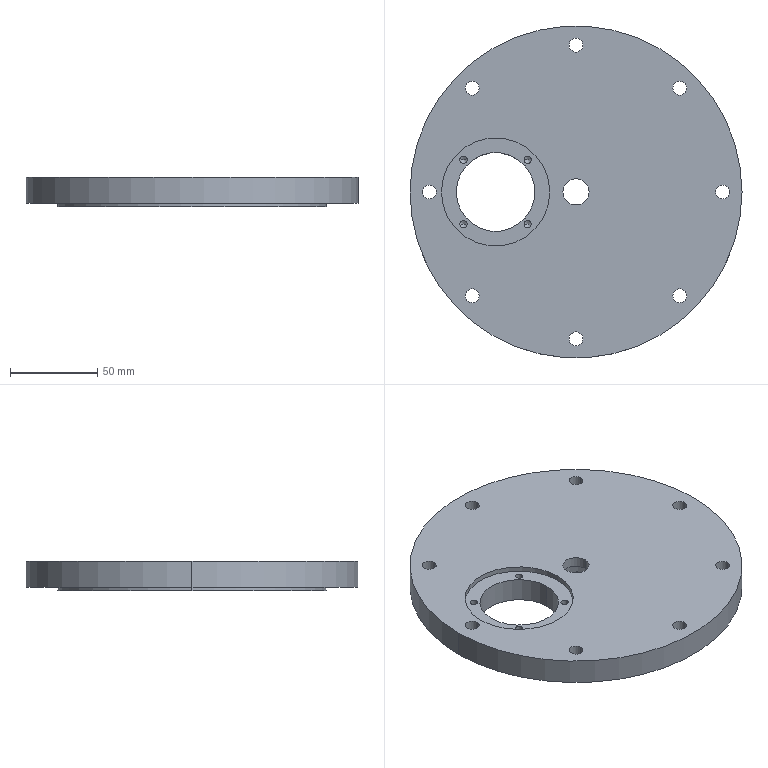Part | SolidWorks | features ICE 4, Cut 2, Extrusion 1, HoleWzd 1 | 1 solid | 49 faces | box 190 x 190 x 17 mm | volume 412970 mm3 | cylinder 36 | cone 8 | plane 5 | commonest cylinder face diameters 8 x16 4.2 x8 15 x2 35 x2 45 x2 62 x2
STEP:
#1=CARTESIAN_POINT('',(-4.,84.,-1484.048));
#2=VERTEX_POINT('',#1);
#3=CARTESIAN_POINT('',(4.,84.,-1484.048));
#4=VERTEX_POINT('',#3);
#5=CARTESIAN_POINT('',(0.,84.,-1484.048));
#6=DIRECTION('',(0.,0.,1.));
#7=DIRECTION('',(1.,0.,0.));
#8=AXIS2_PLACEMENT_3D('',#5,#6,#7);
#9=CIRCLE('',#8,4.);
#10=EDGE_CURVE('',#2,#4,#9,.T.);
#11=ORIENTED_EDGE('',*,*,#10,.F.);
#12=CARTESIAN_POINT('',(-4.,84.,-1469.048));
#13=VERTEX_POINT('',#12);
#14=CARTESIAN_POINT('',(-4.,84.,-1486.048));
#15=DIRECTION('',(0.,0.,1.));
#16=VECTOR('',#15,1000.);
#17=LINE('',#14,#16);
#18=EDGE_CURVE('',#2,#13,#17,.T.);
#19=ORIENTED_EDGE('',*,*,#18,.T.);
#20=CARTESIAN_POINT('',(4.,84.,-1469.048));
#21=VERTEX_POINT('',#20);
#22=CARTESIAN_POINT('',(0.,84.,-1469.048));
#23=DIRECTION('',(0.,0.,1.));
#24=DIRECTION('',(1.,0.,0.));
#25=AXIS2_PLACEMENT_3D('',#22,#23,#24);
#26=CIRCLE('',#25,4.);
#27=EDGE_CURVE('',#13,#21,#26,.T.);
#28=ORIENTED_EDGE('',*,*,#27,.T.);
#29=CARTESIAN_POINT('',(4.,84.,-1486.048));
#30=DIRECTION('',(0.,0.,1.));
#31=VECTOR('',#30,1000.);
#32=LINE('',#29,#31);
#33=EDGE_CURVE('',#4,#21,#32,.T.);
#34=ORIENTED_EDGE('',*,*,#33,.F.);
#35=EDGE_LOOP('',(#11,#19,#28,#34));
#36=FACE_OUTER_BOUND('',#35,.T.);
#37=CARTESIAN_POINT('',(0.,84.,-1486.048));
#38=DIRECTION('',(0.,0.,1.));
#39=DIRECTION('',(1.,0.,0.));
#40=AXIS2_PLACEMENT_3D('',#37,#38,#39);
#41=CYLINDRICAL_SURFACE('',#40,4.);
#42=ADVANCED_FACE('',(#36),#41,.F.);
#43=CARTESIAN_POINT('',(55.397,59.397,-1484.048));
#44=VERTEX_POINT('',#43);
#45=CARTESIAN_POINT('',(63.397,59.397,-1484.048));
#46=VERTEX_POINT('',#45);
#47=CARTESIAN_POINT('',(59.397,59.397,-1484.048));
#48=DIRECTION('',(0.,0.,1.));
#49=DIRECTION('',(1.,0.,0.));
#50=AXIS2_PLACEMENT_3D('',#47,#48,#49);
#51=CIRCLE('',#50,4.);
#52=EDGE_CURVE('',#44,#46,#51,.T.);
#53=ORIENTED_EDGE('',*,*,#52,.F.);
#54=CARTESIAN_POINT('',(55.397,59.397,-1469.048));
#55=VERTEX_POINT('',#54);
#56=CARTESIAN_POINT('',(55.397,59.397,-1486.048));
#57=DIRECTION('',(0.,0.,1.));
#58=VECTOR('',#57,1000.);
#59=LINE('',#56,#58);
#60=EDGE_CURVE('',#44,#55,#59,.T.);
#61=ORIENTED_EDGE('',*,*,#60,.T.);
#62=CARTESIAN_POINT('',(63.397,59.397,-1469.048));
#63=VERTEX_POINT('',#62);
#64=CARTESIAN_POINT('',(59.397,59.397,-1469.048));
#65=DIRECTION('',(0.,0.,1.));
#66=DIRECTION('',(1.,0.,0.));
#67=AXIS2_PLACEMENT_3D('',#64,#65,#66);
#68=CIRCLE('',#67,4.);
#69=EDGE_CURVE('',#55,#63,#68,.T.);
#70=ORIENTED_EDGE('',*,*,#69,.T.);
#71=CARTESIAN_POINT('',(63.397,59.397,-1486.048));
#72=DIRECTION('',(0.,0.,1.));
#73=VECTOR('',#72,1000.);
#74=LINE('',#71,#73);
#75=EDGE_CURVE('',#46,#63,#74,.T.);
#76=ORIENTED_EDGE('',*,*,#75,.F.);
#77=EDGE_LOOP('',(#53,#61,#70,#76));
#78=FACE_OUTER_BOUND('',#77,.T.);
#79=CARTESIAN_POINT('',(59.397,59.397,-1486.048));
#80=DIRECTION('',(0.,0.,1.));
#81=DIRECTION('',(1.,0.,0.));
#82=AXIS2_PLACEMENT_3D('',#79,#80,#81);
#83=CYLINDRICAL_SURFACE('',#82,4.);
#84=ADVANCED_FACE('',(#78),#83,.F.);
#85=CARTESIAN_POINT('',(80.,0.,-1484.048));
#86=VERTEX_POINT('',#85);
#87=CARTESIAN_POINT('',(88.,0.,-1484.048));
#88=VERTEX_POINT('',#87);
#89=CARTESIAN_POINT('',(84.,0.,-1484.048));
#90=DIRECTION('',(0.,0.,1.));
#91=DIRECTION('',(1.,0.,0.));
#92=AXIS2_PLACEMENT_3D('',#89,#90,#91);
#93=CIRCLE('',#92,4.);
#94=EDGE_CURVE('',#86,#88,#93,.T.);
#95=ORIENTED_EDGE('',*,*,#94,.F.);
#96=CARTESIAN_POINT('',(80.,0.,-1469.048));
#97=VERTEX_POINT('',#96);
#98=CARTESIAN_POINT('',(80.,0.,-1486.048));
#99=DIRECTION('',(0.,0.,1.));
#100=VECTOR('',#99,1000.);
#101=LINE('',#98,#100);
#102=EDGE_CURVE('',#86,#97,#101,.T.);
#103=ORIENTED_EDGE('',*,*,#102,.T.);
#104=CARTESIAN_POINT('',(88.,0.,-1469.048));
#105=VERTEX_POINT('',#104);
#106=CARTESIAN_POINT('',(84.,0.,-1469.048));
#107=DIRECTION('',(0.,0.,1.));
#108=DIRECTION('',(1.,0.,0.));
#109=AXIS2_PLACEMENT_3D('',#106,#107,#108);
#110=CIRCLE('',#109,4.);
#111=EDGE_CURVE('',#97,#105,#110,.T.);
#112=ORIENTED_EDGE('',*,*,#111,.T.);
#113=CARTESIAN_POINT('',(88.,0.,-1486.048));
#114=DIRECTION('',(0.,0.,1.));
#115=VECTOR('',#114,1000.);
#116=LINE('',#113,#115);
#117=EDGE_CURVE('',#88,#105,#116,.T.);
#118=ORIENTED_EDGE('',*,*,#117,.F.);
#119=EDGE_LOOP('',(#95,#103,#112,#118));
#120=FACE_OUTER_BOUND('',#119,.T.);
#121=CARTESIAN_POINT('',(84.,0.,-1486.048));
#122=DIRECTION('',(0.,0.,1.));
#123=DIRECTION('',(1.,0.,0.));
#124=AXIS2_PLACEMENT_3D('',#121,#122,#123);
#125=CYLINDRICAL_SURFACE('',#124,4.);
#126=ADVANCED_FACE('',(#120),#125,.F.);
#127=CARTESIAN_POINT('',(55.397,-59.397,-1484.048));
#128=VERTEX_POINT('',#127);
#129=CARTESIAN_POINT('',(63.397,-59.397,-1484.048));
#130=VERTEX_POINT('',#129);
#131=CARTESIAN_POINT('',(59.397,-59.397,-1484.048));
#132=DIRECTION('',(0.,0.,1.));
#133=DIRECTION('',(1.,0.,0.));
#134=AXIS2_PLACEMENT_3D('',#131,#132,#133);
#135=CIRCLE('',#134,4.);
#136=EDGE_CURVE('',#128,#130,#135,.T.);
#137=ORIENTED_EDGE('',*,*,#136,.F.);
#138=CARTESIAN_POINT('',(55.397,-59.397,-1469.048));
#139=VERTEX_POINT('',#138);
#140=CARTESIAN_POINT('',(55.397,-59.397,-1486.048));
#141=DIRECTION('',(0.,0.,1.));
#142=VECTOR('',#141,1000.);
#143=LINE('',#140,#142);
#144=EDGE_CURVE('',#128,#139,#143,.T.);
#145=ORIENTED_EDGE('',*,*,#144,.T.);
#146=CARTESIAN_POINT('',(63.397,-59.397,-1469.048));
#147=VERTEX_POINT('',#146);
#148=CARTESIAN_POINT('',(59.397,-59.397,-1469.048));
#149=DIRECTION('',(0.,0.,1.));
#150=DIRECTION('',(1.,0.,0.));
#151=AXIS2_PLACEMENT_3D('',#148,#149,#150);
#152=CIRCLE('',#151,4.);
#153=EDGE_CURVE('',#139,#147,#152,.T.);
#154=ORIENTED_EDGE('',*,*,#153,.T.);
#155=CARTESIAN_POINT('',(63.397,-59.397,-1486.048));
#156=DIRECTION('',(0.,0.,1.));
#157=VECTOR('',#156,1000.);
#158=LINE('',#155,#157);
#159=EDGE_CURVE('',#130,#147,#158,.T.);
#160=ORIENTED_EDGE('',*,*,#159,.F.);
#161=EDGE_LOOP('',(#137,#145,#154,#160));
#162=FACE_OUTER_BOUND('',#161,.T.);
#163=CARTESIAN_POINT('',(59.397,-59.397,-1486.048));
#164=DIRECTION('',(0.,0.,1.));
#165=DIRECTION('',(1.,0.,0.));
#166=AXIS2_PLACEMENT_3D('',#163,#164,#165);
#167=CYLINDRICAL_SURFACE('',#166,4.);
#168=ADVANCED_FACE('',(#162),#167,.F.);
#169=CARTESIAN_POINT('',(-4.,-84.,-1484.048));
#170=VERTEX_POINT('',#169);
#171=CARTESIAN_POINT('',(4.,-84.,-1484.048));
#172=VERTEX_POINT('',#171);
#173=CARTESIAN_POINT('',(0.,-84.,-1484.048));
#174=DIRECTION('',(0.,0.,1.));
#175=DIRECTION('',(1.,0.,0.));
#176=AXIS2_PLACEMENT_3D('',#173,#174,#175);
#177=CIRCLE('',#176,4.);
#178=EDGE_CURVE('',#170,#172,#177,.T.);
#179=ORIENTED_EDGE('',*,*,#178,.F.);
#180=CARTESIAN_POINT('',(-4.,-84.,-1469.048));
#181=VERTEX_POINT('',#180);
#182=CARTESIAN_POINT('',(-4.,-84.,-1486.048));
#183=DIRECTION('',(0.,0.,1.));
#184=VECTOR('',#183,1000.);
#185=LINE('',#182,#184);
#186=EDGE_CURVE('',#170,#181,#185,.T.);
#187=ORIENTED_EDGE('',*,*,#186,.T.);
#188=CARTESIAN_POINT('',(4.,-84.,-1469.048));
#189=VERTEX_POINT('',#188);
#190=CARTESIAN_POINT('',(0.,-84.,-1469.048));
#191=DIRECTION('',(0.,0.,1.));
#192=DIRECTION('',(1.,0.,0.));
#193=AXIS2_PLACEMENT_3D('',#190,#191,#192);
#194=CIRCLE('',#193,4.);
#195=EDGE_CURVE('',#181,#189,#194,.T.);
#196=ORIENTED_EDGE('',*,*,#195,.T.);
#197=CARTESIAN_POINT('',(4.,-84.,-1486.048));
#198=DIRECTION('',(0.,0.,1.));
#199=VECTOR('',#198,1000.);
#200=LINE('',#197,#199);
#201=EDGE_CURVE('',#172,#189,#200,.T.);
#202=ORIENTED_EDGE('',*,*,#201,.F.);
#203=EDGE_LOOP('',(#179,#187,#196,#202));
#204=FACE_OUTER_BOUND('',#203,.T.);
#205=CARTESIAN_POINT('',(0.,-84.,-1486.048));
#206=DIRECTION('',(0.,0.,1.));
#207=DIRECTION('',(1.,0.,0.));
#208=AXIS2_PLACEMENT_3D('',#205,#206,#207);
#209=CYLINDRICAL_SURFACE('',#208,4.);
#210=ADVANCED_FACE('',(#204),#209,.F.);
#211=CARTESIAN_POINT('',(-63.397,-59.397,-1484.048));
#212=VERTEX_POINT('',#211);
#213=CARTESIAN_POINT('',(-55.397,-59.397,-1484.048));
#214=VERTEX_POINT('',#213);
#215=CARTESIAN_POINT('',(-59.397,-59.397,-1484.048));
#216=DIRECTION('',(0.,0.,1.));
#217=DIRECTION('',(1.,0.,0.));
#218=AXIS2_PLACEMENT_3D('',#215,#216,#217);
#219=CIRCLE('',#218,4.);
#220=EDGE_CURVE('',#212,#214,#219,.T.);
#221=ORIENTED_EDGE('',*,*,#220,.F.);
#222=CARTESIAN_POINT('',(-63.397,-59.397,-1469.048));
#223=VERTEX_POINT('',#222);
#224=CARTESIAN_POINT('',(-63.397,-59.397,-1486.048));
#225=DIRECTION('',(0.,0.,1.));
#226=VECTOR('',#225,1000.);
#227=LINE('',#224,#226);
#228=EDGE_CURVE('',#212,#223,#227,.T.);
#229=ORIENTED_EDGE('',*,*,#228,.T.);
#230=CARTESIAN_POINT('',(-55.397,-59.397,-1469.048));
#231=VERTEX_POINT('',#230);
#232=CARTESIAN_POINT('',(-59.397,-59.397,-1469.048));
#233=DIRECTION('',(0.,0.,1.));
#234=DIRECTION('',(1.,0.,0.));
#235=AXIS2_PLACEMENT_3D('',#232,#233,#234);
#236=CIRCLE('',#235,4.);
#237=EDGE_CURVE('',#223,#231,#236,.T.);
#238=ORIENTED_EDGE('',*,*,#237,.T.);
#239=CARTESIAN_POINT('',(-55.397,-59.397,-1486.048));
#240=DIRECTION('',(0.,0.,1.));
#241=VECTOR('',#240,1000.);
#242=LINE('',#239,#241);
#243=EDGE_CURVE('',#214,#231,#242,.T.);
#244=ORIENTED_EDGE('',*,*,#243,.F.);
#245=EDGE_LOOP('',(#221,#229,#238,#244));
#246=FACE_OUTER_BOUND('',#245,.T.);
#247=CARTESIAN_POINT('',(-59.397,-59.397,-1486.048));
#248=DIRECTION('',(0.,0.,1.));
#249=DIRECTION('',(1.,0.,0.));
#250=AXIS2_PLACEMENT_3D('',#247,#248,#249);
#251=CYLINDRICAL_SURFACE('',#250,4.);
#252=ADVANCED_FACE('',(#246),#251,.F.);
#253=CARTESIAN_POINT('',(-88.,0.,-1484.048));
#254=VERTEX_POINT('',#253);
#255=CARTESIAN_POINT('',(-80.,0.,-1484.048));
#256=VERTEX_POINT('',#255);
#257=CARTESIAN_POINT('',(-84.,0.,-1484.048));
#258=DIRECTION('',(0.,0.,1.));
#259=DIRECTION('',(1.,0.,0.));
#260=AXIS2_PLACEMENT_3D('',#257,#258,#259);
#261=CIRCLE('',#260,4.);
#262=EDGE_CURVE('',#254,#256,#261,.T.);
#263=ORIENTED_EDGE('',*,*,#262,.F.);
#264=CARTESIAN_POINT('',(-88.,0.,-1469.048));
#265=VERTEX_POINT('',#264);
#266=CARTESIAN_POINT('',(-88.,0.,-1486.048));
#267=DIRECTION('',(0.,0.,1.));
#268=VECTOR('',#267,1000.);
#269=LINE('',#266,#268);
#270=EDGE_CURVE('',#254,#265,#269,.T.);
#271=ORIENTED_EDGE('',*,*,#270,.T.);
#272=CARTESIAN_POINT('',(-80.,0.,-1469.048));
#273=VERTEX_POINT('',#272);
#274=CARTESIAN_POINT('',(-84.,0.,-1469.048));
#275=DIRECTION('',(0.,0.,1.));
#276=DIRECTION('',(1.,0.,0.));
#277=AXIS2_PLACEMENT_3D('',#274,#275,#276);
#278=CIRCLE('',#277,4.);
#279=EDGE_CURVE('',#265,#273,#278,.T.);
#280=ORIENTED_EDGE('',*,*,#279,.T.);
#281=CARTESIAN_POINT('',(-80.,0.,-1486.048));
#282=DIRECTION('',(0.,0.,1.));
#283=VECTOR('',#282,1000.);
#284=LINE('',#281,#283);
#285=EDGE_CURVE('',#256,#273,#284,.T.);
#286=ORIENTED_EDGE('',*,*,#285,.F.);
#287=EDGE_LOOP('',(#263,#271,#280,#286));
#288=FACE_OUTER_BOUND('',#287,.T.);
#289=CARTESIAN_POINT('',(-84.,0.,-1486.048));
#290=DIRECTION('',(0.,0.,1.));
#291=DIRECTION('',(1.,0.,0.));
#292=AXIS2_PLACEMENT_3D('',#289,#290,#291);
#293=CYLINDRICAL_SURFACE('',#292,4.);
#294=ADVANCED_FACE('',(#288),#293,.F.);
#295=CARTESIAN_POINT('',(-63.397,59.397,-1484.048));
#296=VERTEX_POINT('',#295);
#297=CARTESIAN_POINT('',(-55.397,59.397,-1484.048));
#298=VERTEX_POINT('',#297);
#299=CARTESIAN_POINT('',(-59.397,59.397,-1484.048));
#300=DIRECTION('',(0.,0.,1.));
#301=DIRECTION('',(1.,0.,0.));
#302=AXIS2_PLACEMENT_3D('',#299,#300,#301);
#303=CIRCLE('',#302,4.);
#304=EDGE_CURVE('',#296,#298,#303,.T.);
#305=ORIENTED_EDGE('',*,*,#304,.F.);
#306=CARTESIAN_POINT('',(-63.397,59.397,-1469.048));
#307=VERTEX_POINT('',#306);
#308=CARTESIAN_POINT('',(-63.397,59.397,-1486.048));
#309=DIRECTION('',(0.,0.,1.));
#310=VECTOR('',#309,1000.);
#311=LINE('',#308,#310);
#312=EDGE_CURVE('',#296,#307,#311,.T.);
#313=ORIENTED_EDGE('',*,*,#312,.T.);
#314=CARTESIAN_POINT('',(-55.397,59.397,-1469.048));
#315=VERTEX_POINT('',#314);
#316=CARTESIAN_POINT('',(-59.397,59.397,-1469.048));
#317=DIRECTION('',(0.,0.,1.));
#318=DIRECTION('',(1.,0.,0.));
#319=AXIS2_PLACEMENT_3D('',#316,#317,#318);
#320=CIRCLE('',#319,4.);
#321=EDGE_CURVE('',#307,#315,#320,.T.);
#322=ORIENTED_EDGE('',*,*,#321,.T.);
#323=CARTESIAN_POINT('',(-55.397,59.397,-1486.048));
#324=DIRECTION('',(0.,0.,1.));
#325=VECTOR('',#324,1000.);
#326=LINE('',#323,#325);
#327=EDGE_CURVE('',#298,#315,#326,.T.);
#328=ORIENTED_EDGE('',*,*,#327,.F.);
#329=EDGE_LOOP('',(#305,#313,#322,#328));
#330=FACE_OUTER_BOUND('',#329,.T.);
#331=CARTESIAN_POINT('',(-59.397,59.397,-1486.048));
#332=DIRECTION('',(0.,0.,1.));
#333=DIRECTION('',(1.,0.,0.));
#334=AXIS2_PLACEMENT_3D('',#331,#332,#333);
#335=CYLINDRICAL_SURFACE('',#334,4.);
#336=ADVANCED_FACE('',(#330),#335,.F.);
#337=CARTESIAN_POINT('',(-29.715,18.385,-1482.048));
#338=VERTEX_POINT('',#337);
#339=CARTESIAN_POINT('',(-25.515,18.385,-1482.048));
#340=VERTEX_POINT('',#339);
#341=CARTESIAN_POINT('',(-27.615,18.385,-1482.048));
#342=DIRECTION('',(0.,0.,1.));
#343=DIRECTION('',(1.,0.,0.));
#344=AXIS2_PLACEMENT_3D('',#341,#342,#343);
#345=CIRCLE('',#344,2.1);
#346=EDGE_CURVE('',#338,#340,#345,.T.);
#347=ORIENTED_EDGE('',*,*,#346,.F.);
#348=CARTESIAN_POINT('',(-29.715,18.385,-1472.048));
#349=VERTEX_POINT('',#348);
#350=CARTESIAN_POINT('',(-29.715,18.385,-1472.048));
#351=DIRECTION('',(0.,0.,1.));
#352=VECTOR('',#351,1000.);
#353=LINE('',#350,#352);
#354=EDGE_CURVE('',#338,#349,#353,.T.);
#355=ORIENTED_EDGE('',*,*,#354,.T.);
#356=CARTESIAN_POINT('',(-25.515,18.385,-1472.048));
#357=VERTEX_POINT('',#356);
#358=CARTESIAN_POINT('',(-27.615,18.385,-1472.048));
#359=DIRECTION('',(0.,0.,1.));
#360=DIRECTION('',(1.,0.,0.));
#361=AXIS2_PLACEMENT_3D('',#358,#359,#360);
#362=CIRCLE('',#361,2.1);
#363=EDGE_CURVE('',#349,#357,#362,.T.);
#364=ORIENTED_EDGE('',*,*,#363,.T.);
#365=CARTESIAN_POINT('',(-25.515,18.385,-1472.048));
#366=DIRECTION('',(0.,0.,1.));
#367=VECTOR('',#366,1000.);
#368=LINE('',#365,#367);
#369=EDGE_CURVE('',#340,#357,#368,.T.);
#370=ORIENTED_EDGE('',*,*,#369,.F.);
#371=EDGE_LOOP('',(#347,#355,#364,#370));
#372=FACE_OUTER_BOUND('',#371,.T.);
#373=CARTESIAN_POINT('',(-27.615,18.385,-1472.048));
#374=DIRECTION('',(0.,0.,1.));
#375=DIRECTION('',(1.,0.,0.));
#376=AXIS2_PLACEMENT_3D('',#373,#374,#375);
#377=CYLINDRICAL_SURFACE('',#376,2.1);
#378=ADVANCED_FACE('',(#372),#377,.F.);
#379=CARTESIAN_POINT('',(-27.615,18.385,-1483.31));
#380=VERTEX_POINT('',#379);
#381=CARTESIAN_POINT('',(-25.515,18.385,-1482.048));
#382=DIRECTION('',(0.8572,0.,0.515));
#383=VECTOR('',#382,1000.);
#384=LINE('',#381,#383);
#385=EDGE_CURVE('',#380,#340,#384,.T.);
#386=ORIENTED_EDGE('',*,*,#385,.F.);
#387=CARTESIAN_POINT('',(-29.715,18.385,-1482.048));
#388=DIRECTION('',(-0.8572,0.,0.515));
#389=VECTOR('',#388,1000.);
#390=LINE('',#387,#389);
#391=EDGE_CURVE('',#380,#338,#390,.T.);
#392=ORIENTED_EDGE('',*,*,#391,.T.);
#393=ORIENTED_EDGE('',*,*,#346,.T.);
#394=EDGE_LOOP('',(#386,#392,#393));
#395=FACE_OUTER_BOUND('',#394,.T.);
#396=CARTESIAN_POINT('',(-27.615,18.385,-1482.048));
#397=DIRECTION('',(0.,0.,1.));
#398=DIRECTION('',(1.,0.,0.));
#399=AXIS2_PLACEMENT_3D('',#396,#397,#398);
#400=CONICAL_SURFACE('',#399,2.1,1.03);
#401=ADVANCED_FACE('',(#395),#400,.F.);
#402=CARTESIAN_POINT('',(-29.715,-18.385,-1482.048));
#403=VERTEX_POINT('',#402);
#404=CARTESIAN_POINT('',(-25.515,-18.385,-1482.048));
#405=VERTEX_POINT('',#404);
#406=CARTESIAN_POINT('',(-27.615,-18.385,-1482.048));
#407=DIRECTION('',(0.,0.,1.));
#408=DIRECTION('',(1.,0.,0.));
#409=AXIS2_PLACEMENT_3D('',#406,#407,#408);
#410=CIRCLE('',#409,2.1);
#411=EDGE_CURVE('',#403,#405,#410,.T.);
#412=ORIENTED_EDGE('',*,*,#411,.F.);
#413=CARTESIAN_POINT('',(-29.715,-18.385,-1472.048));
#414=VERTEX_POINT('',#413);
#415=CARTESIAN_POINT('',(-29.715,-18.385,-1472.048));
#416=DIRECTION('',(0.,0.,1.));
#417=VECTOR('',#416,1000.);
#418=LINE('',#415,#417);
#419=EDGE_CURVE('',#403,#414,#418,.T.);
#420=ORIENTED_EDGE('',*,*,#419,.T.);
#421=CARTESIAN_POINT('',(-25.515,-18.385,-1472.048));
#422=VERTEX_POINT('',#421);
#423=CARTESIAN_POINT('',(-27.615,-18.385,-1472.048));
#424=DIRECTION('',(0.,0.,1.));
#425=DIRECTION('',(1.,0.,0.));
#426=AXIS2_PLACEMENT_3D('',#423,#424,#425);
#427=CIRCLE('',#426,2.1);
#428=EDGE_CURVE('',#414,#422,#427,.T.);
#429=ORIENTED_EDGE('',*,*,#428,.T.);
#430=CARTESIAN_POINT('',(-25.515,-18.385,-1472.048));
#431=DIRECTION('',(0.,0.,1.));
#432=VECTOR('',#431,1000.);
#433=LINE('',#430,#432);
#434=EDGE_CURVE('',#405,#422,#433,.T.);
#435=ORIENTED_EDGE('',*,*,#434,.F.);
#436=EDGE_LOOP('',(#412,#420,#429,#435));
#437=FACE_OUTER_BOUND('',#436,.T.);
#438=CARTESIAN_POINT('',(-27.615,-18.385,-1472.048));
#439=DIRECTION('',(0.,0.,1.));
#440=DIRECTION('',(1.,0.,0.));
#441=AXIS2_PLACEMENT_3D('',#438,#439,#440);
#442=CYLINDRICAL_SURFACE('',#441,2.1);
#443=ADVANCED_FACE('',(#437),#442,.F.);
#444=CARTESIAN_POINT('',(-27.615,-18.385,-1483.31));
#445=VERTEX_POINT('',#444);
#446=CARTESIAN_POINT('',(-25.515,-18.385,-1482.048));
#447=DIRECTION('',(0.8572,0.,0.515));
#448=VECTOR('',#447,1000.);
#449=LINE('',#446,#448);
#450=EDGE_CURVE('',#445,#405,#449,.T.);
#451=ORIENTED_EDGE('',*,*,#450,.F.);
#452=CARTESIAN_POINT('',(-29.715,-18.385,-1482.048));
#453=DIRECTION('',(-0.8572,0.,0.515));
#454=VECTOR('',#453,1000.);
#455=LINE('',#452,#454);
#456=EDGE_CURVE('',#445,#403,#455,.T.);
#457=ORIENTED_EDGE('',*,*,#456,.T.);
#458=ORIENTED_EDGE('',*,*,#411,.T.);
#459=EDGE_LOOP('',(#451,#457,#458));
#460=FACE_OUTER_BOUND('',#459,.T.);
#461=CARTESIAN_POINT('',(-27.615,-18.385,-1482.048));
#462=DIRECTION('',(0.,0.,1.));
#463=DIRECTION('',(1.,0.,0.));
#464=AXIS2_PLACEMENT_3D('',#461,#462,#463);
#465=CONICAL_SURFACE('',#464,2.1,1.03);
#466=ADVANCED_FACE('',(#460),#465,.F.);
#467=CARTESIAN_POINT('',(-66.485,-18.385,-1482.048));
#468=VERTEX_POINT('',#467);
#469=CARTESIAN_POINT('',(-62.285,-18.385,-1482.048));
#470=VERTEX_POINT('',#469);
#471=CARTESIAN_POINT('',(-64.385,-18.385,-1482.048));
#472=DIRECTION('',(0.,0.,1.));
#473=DIRECTION('',(1.,0.,0.));
#474=AXIS2_PLACEMENT_3D('',#471,#472,#473);
#475=CIRCLE('',#474,2.1);
#476=EDGE_CURVE('',#468,#470,#475,.T.);
#477=ORIENTED_EDGE('',*,*,#476,.F.);
#478=CARTESIAN_POINT('',(-66.485,-18.385,-1472.048));
#479=VERTEX_POINT('',#478);
#480=CARTESIAN_POINT('',(-66.485,-18.385,-1472.048));
#481=DIRECTION('',(0.,0.,1.));
#482=VECTOR('',#481,1000.);
#483=LINE('',#480,#482);
#484=EDGE_CURVE('',#468,#479,#483,.T.);
#485=ORIENTED_EDGE('',*,*,#484,.T.);
#486=CARTESIAN_POINT('',(-62.285,-18.385,-1472.048));
#487=VERTEX_POINT('',#486);
#488=CARTESIAN_POINT('',(-64.385,-18.385,-1472.048));
#489=DIRECTION('',(0.,0.,1.));
#490=DIRECTION('',(1.,0.,0.));
#491=AXIS2_PLACEMENT_3D('',#488,#489,#490);
#492=CIRCLE('',#491,2.1);
#493=EDGE_CURVE('',#479,#487,#492,.T.);
#494=ORIENTED_EDGE('',*,*,#493,.T.);
#495=CARTESIAN_POINT('',(-62.285,-18.385,-1472.048));
#496=DIRECTION('',(0.,0.,1.));
#497=VECTOR('',#496,1000.);
#498=LINE('',#495,#497);
#499=EDGE_CURVE('',#470,#487,#498,.T.);
#500=ORIENTED_EDGE('',*,*,#499,.F.);
#501=EDGE_LOOP('',(#477,#485,#494,#500));
#502=FACE_OUTER_BOUND('',#501,.T.);
#503=CARTESIAN_POINT('',(-64.385,-18.385,-1472.048));
#504=DIRECTION('',(0.,0.,1.));
#505=DIRECTION('',(1.,0.,0.));
#506=AXIS2_PLACEMENT_3D('',#503,#504,#505);
#507=CYLINDRICAL_SURFACE('',#506,2.1);
#508=ADVANCED_FACE('',(#502),#507,.F.);
#509=CARTESIAN_POINT('',(-64.385,-18.385,-1483.31));
#510=VERTEX_POINT('',#509);
#511=CARTESIAN_POINT('',(-62.285,-18.385,-1482.048));
#512=DIRECTION('',(0.8572,0.,0.515));
#513=VECTOR('',#512,1000.);
#514=LINE('',#511,#513);
#515=EDGE_CURVE('',#510,#470,#514,.T.);
#516=ORIENTED_EDGE('',*,*,#515,.F.);
#517=CARTESIAN_POINT('',(-66.485,-18.385,-1482.048));
#518=DIRECTION('',(-0.8572,0.,0.515));
#519=VECTOR('',#518,1000.);
#520=LINE('',#517,#519);
#521=EDGE_CURVE('',#510,#468,#520,.T.);
#522=ORIENTED_EDGE('',*,*,#521,.T.);
#523=ORIENTED_EDGE('',*,*,#476,.T.);
#524=EDGE_LOOP('',(#516,#522,#523));
#525=FACE_OUTER_BOUND('',#524,.T.);
#526=CARTESIAN_POINT('',(-64.385,-18.385,-1482.048));
#527=DIRECTION('',(0.,0.,1.));
#528=DIRECTION('',(1.,0.,0.));
#529=AXIS2_PLACEMENT_3D('',#526,#527,#528);
#530=CONICAL_SURFACE('',#529,2.1,1.03);
#531=ADVANCED_FACE('',(#525),#530,.F.);
#532=CARTESIAN_POINT('',(-66.485,18.385,-1482.048));
#533=VERTEX_POINT('',#532);
#534=CARTESIAN_POINT('',(-62.285,18.385,-1482.048));
#535=VERTEX_POINT('',#534);
#536=CARTESIAN_POINT('',(-64.385,18.385,-1482.048));
#537=DIRECTION('',(0.,0.,1.));
#538=DIRECTION('',(1.,0.,0.));
#539=AXIS2_PLACEMENT_3D('',#536,#537,#538);
#540=CIRCLE('',#539,2.1);
#541=EDGE_CURVE('',#533,#535,#540,.T.);
#542=ORIENTED_EDGE('',*,*,#541,.F.);
#543=CARTESIAN_POINT('',(-66.485,18.385,-1472.048));
#544=VERTEX_POINT('',#543);
#545=CARTESIAN_POINT('',(-66.485,18.385,-1472.048));
#546=DIRECTION('',(0.,0.,1.));
#547=VECTOR('',#546,1000.);
#548=LINE('',#545,#547);
#549=EDGE_CURVE('',#533,#544,#548,.T.);
#550=ORIENTED_EDGE('',*,*,#549,.T.);
#551=CARTESIAN_POINT('',(-62.285,18.385,-1472.048));
#552=VERTEX_POINT('',#551);
#553=CARTESIAN_POINT('',(-64.385,18.385,-1472.048));
#554=DIRECTION('',(0.,0.,1.));
#555=DIRECTION('',(1.,0.,0.));
#556=AXIS2_PLACEMENT_3D('',#553,#554,#555);
#557=CIRCLE('',#556,2.1);
#558=EDGE_CURVE('',#544,#552,#557,.T.);
#559=ORIENTED_EDGE('',*,*,#558,.T.);
#560=CARTESIAN_POINT('',(-62.285,18.385,-1472.048));
#561=DIRECTION('',(0.,0.,1.));
#562=VECTOR('',#561,1000.);
#563=LINE('',#560,#562);
#564=EDGE_CURVE('',#535,#552,#563,.T.);
#565=ORIENTED_EDGE('',*,*,#564,.F.);
#566=EDGE_LOOP('',(#542,#550,#559,#565));
#567=FACE_OUTER_BOUND('',#566,.T.);
#568=CARTESIAN_POINT('',(-64.385,18.385,-1472.048));
#569=DIRECTION('',(0.,0.,1.));
#570=DIRECTION('',(1.,0.,0.));
#571=AXIS2_PLACEMENT_3D('',#568,#569,#570);
#572=CYLINDRICAL_SURFACE('',#571,2.1);
#573=ADVANCED_FACE('',(#567),#572,.F.);
#574=CARTESIAN_POINT('',(-64.385,18.385,-1483.31));
#575=VERTEX_POINT('',#574);
#576=CARTESIAN_POINT('',(-62.285,18.385,-1482.048));
#577=DIRECTION('',(0.8572,0.,0.515));
#578=VECTOR('',#577,1000.);
#579=LINE('',#576,#578);
#580=EDGE_CURVE('',#575,#535,#579,.T.);
#581=ORIENTED_EDGE('',*,*,#580,.F.);
#582=CARTESIAN_POINT('',(-66.485,18.385,-1482.048));
#583=DIRECTION('',(-0.8572,0.,0.515));
#584=VECTOR('',#583,1000.);
#585=LINE('',#582,#584);
#586=EDGE_CURVE('',#575,#533,#585,.T.);
#587=ORIENTED_EDGE('',*,*,#586,.T.);
#588=ORIENTED_EDGE('',*,*,#541,.T.);
#589=EDGE_LOOP('',(#581,#587,#588));
#590=FACE_OUTER_BOUND('',#589,.T.);
#591=CARTESIAN_POINT('',(-64.385,18.385,-1482.048));
#592=DIRECTION('',(0.,0.,1.));
#593=DIRECTION('',(1.,0.,0.));
#594=AXIS2_PLACEMENT_3D('',#591,#592,#593);
#595=CONICAL_SURFACE('',#594,2.1,1.03);
#596=ADVANCED_FACE('',(#590),#595,.F.);
#597=CARTESIAN_POINT('',(-77.,0.,-1472.048));
#598=VERTEX_POINT('',#597);
#599=CARTESIAN_POINT('',(-15.,0.,-1472.048));
#600=VERTEX_POINT('',#599);
#601=CARTESIAN_POINT('',(-46.,0.,-1472.048));
#602=DIRECTION('',(0.,0.,1.));
#603=DIRECTION('',(1.,0.,0.));
#604=AXIS2_PLACEMENT_3D('',#601,#602,#603);
#605=CIRCLE('',#604,31.);
#606=EDGE_CURVE('',#598,#600,#605,.T.);
#607=ORIENTED_EDGE('',*,*,#606,.F.);
#608=CARTESIAN_POINT('',(-77.,0.,-1469.048));
#609=VERTEX_POINT('',#608);
#610=CARTESIAN_POINT('',(-77.,0.,-1472.048));
#611=DIRECTION('',(0.,0.,1.));
#612=VECTOR('',#611,1000.);
#613=LINE('',#610,#612);
#614=EDGE_CURVE('',#598,#609,#613,.T.);
#615=ORIENTED_EDGE('',*,*,#614,.T.);
#616=CARTESIAN_POINT('',(-15.,0.,-1469.048));
#617=VERTEX_POINT('',#616);
#618=CARTESIAN_POINT('',(-46.,0.,-1469.048));
#619=DIRECTION('',(0.,0.,1.));
#620=DIRECTION('',(1.,0.,0.));
#621=AXIS2_PLACEMENT_3D('',#618,#619,#620);
#622=CIRCLE('',#621,31.);
#623=EDGE_CURVE('',#609,#617,#622,.T.);
#624=ORIENTED_EDGE('',*,*,#623,.T.);
#625=CARTESIAN_POINT('',(-15.,0.,-1472.048));
#626=DIRECTION('',(0.,0.,1.));
#627=VECTOR('',#626,1000.);
#628=LINE('',#625,#627);
#629=EDGE_CURVE('',#600,#617,#628,.T.);
#630=ORIENTED_EDGE('',*,*,#629,.F.);
#631=EDGE_LOOP('',(#607,#615,#624,#630));
#632=FACE_OUTER_BOUND('',#631,.T.);
#633=CARTESIAN_POINT('',(-46.,0.,-1472.048));
#634=DIRECTION('',(0.,0.,1.));
#635=DIRECTION('',(1.,0.,0.));
#636=AXIS2_PLACEMENT_3D('',#633,#634,#635);
#637=CYLINDRICAL_SURFACE('',#636,31.);
#638=ADVANCED_FACE('',(#632),#637,.F.);
#639=CARTESIAN_POINT('',(-7.5,0.,-1469.048));
#640=VERTEX_POINT('',#639);
#641=CARTESIAN_POINT('',(7.5,0.,-1469.048));
#642=VERTEX_POINT('',#641);
#643=CARTESIAN_POINT('',(0.,0.,-1469.048));
#644=DIRECTION('',(0.,0.,1.));
#645=DIRECTION('',(1.,0.,0.));
#646=AXIS2_PLACEMENT_3D('',#643,#644,#645);
#647=CIRCLE('',#646,7.5);
#648=EDGE_CURVE('',#640,#642,#647,.T.);
#649=ORIENTED_EDGE('',*,*,#648,.T.);
#650=CARTESIAN_POINT('',(7.5,0.,-1475.048));
#651=VERTEX_POINT('',#650);
#652=CARTESIAN_POINT('',(7.5,0.,-1463.048));
#653=DIRECTION('',(0.,0.,-1.));
#654=VECTOR('',#653,1000.);
#655=LINE('',#652,#654);
#656=EDGE_CURVE('',#642,#651,#655,.T.);
#657=ORIENTED_EDGE('',*,*,#656,.T.);
#658=CARTESIAN_POINT('',(-7.5,0.,-1475.048));
#659=VERTEX_POINT('',#658);
#660=CARTESIAN_POINT('',(0.,0.,-1475.048));
#661=DIRECTION('',(0.,0.,-1.));
#662=DIRECTION('',(-1.,0.,0.));
#663=AXIS2_PLACEMENT_3D('',#660,#661,#662);
#664=CIRCLE('',#663,7.5);
#665=EDGE_CURVE('',#651,#659,#664,.T.);
#666=ORIENTED_EDGE('',*,*,#665,.T.);
#667=CARTESIAN_POINT('',(-7.5,0.,-1463.048));
#668=DIRECTION('',(0.,0.,-1.));
#669=VECTOR('',#668,1000.);
#670=LINE('',#667,#669);
#671=EDGE_CURVE('',#640,#659,#670,.T.);
#672=ORIENTED_EDGE('',*,*,#671,.F.);
#673=EDGE_LOOP('',(#649,#657,#666,#672));
#674=FACE_OUTER_BOUND('',#673,.T.);
#675=CARTESIAN_POINT('',(0.,0.,-1463.048));
#676=DIRECTION('',(0.,0.,-1.));
#677=DIRECTION('',(-1.,0.,0.));
#678=AXIS2_PLACEMENT_3D('',#675,#676,#677);
#679=CYLINDRICAL_SURFACE('',#678,7.5);
#680=ADVANCED_FACE('',(#674),#679,.F.);
#681=CARTESIAN_POINT('',(17.5,0.,-1475.048));
#682=VERTEX_POINT('',#681);
#683=CARTESIAN_POINT('',(-17.5,0.,-1475.048));
#684=VERTEX_POINT('',#683);
#685=CARTESIAN_POINT('',(0.,0.,-1475.048));
#686=DIRECTION('',(0.,0.,-1.));
#687=DIRECTION('',(-1.,0.,0.));
#688=AXIS2_PLACEMENT_3D('',#685,#686,#687);
#689=CIRCLE('',#688,17.5);
#690=EDGE_CURVE('',#682,#684,#689,.T.);
#691=ORIENTED_EDGE('',*,*,#690,.F.);
#692=CARTESIAN_POINT('',(17.5,0.,-1486.048));
#693=VERTEX_POINT('',#692);
#694=CARTESIAN_POINT('',(17.5,0.,-1475.048));
#695=DIRECTION('',(0.,0.,-1.));
#696=VECTOR('',#695,1000.);
#697=LINE('',#694,#696);
#698=EDGE_CURVE('',#682,#693,#697,.T.);
#699=ORIENTED_EDGE('',*,*,#698,.T.);
#700=CARTESIAN_POINT('',(-17.5,0.,-1486.048));
#701=VERTEX_POINT('',#700);
#702=CARTESIAN_POINT('',(0.,0.,-1486.048));
#703=DIRECTION('',(0.,0.,-1.));
#704=DIRECTION('',(-1.,0.,0.));
#705=AXIS2_PLACEMENT_3D('',#702,#703,#704);
#706=CIRCLE('',#705,17.5);
#707=EDGE_CURVE('',#693,#701,#706,.T.);
#708=ORIENTED_EDGE('',*,*,#707,.T.);
#709=CARTESIAN_POINT('',(-17.5,0.,-1475.048));
#710=DIRECTION('',(0.,0.,-1.));
#711=VECTOR('',#710,1000.);
#712=LINE('',#709,#711);
#713=EDGE_CURVE('',#684,#701,#712,.T.);
#714=ORIENTED_EDGE('',*,*,#713,.F.);
#715=EDGE_LOOP('',(#691,#699,#708,#714));
#716=FACE_OUTER_BOUND('',#715,.T.);
#717=CARTESIAN_POINT('',(0.,0.,-1475.048));
#718=DIRECTION('',(0.,0.,-1.));
#719=DIRECTION('',(-1.,0.,0.));
#720=AXIS2_PLACEMENT_3D('',#717,#718,#719);
#721=CYLINDRICAL_SURFACE('',#720,17.5);
#722=ADVANCED_FACE('',(#716),#721,.F.);
#723=CARTESIAN_POINT('',(-77.,0.,-1486.048));
#724=VERTEX_POINT('',#723);
#725=CARTESIAN_POINT('',(77.,0.,-1486.048));
#726=VERTEX_POINT('',#725);
#727=CARTESIAN_POINT('',(0.,0.,-1486.048));
#728=DIRECTION('',(0.,0.,-1.));
#729=DIRECTION('',(-1.,0.,0.));
#730=AXIS2_PLACEMENT_3D('',#727,#728,#729);
#731=CIRCLE('',#730,77.);
#732=EDGE_CURVE('',#724,#726,#731,.T.);
#733=ORIENTED_EDGE('',*,*,#732,.F.);
#734=CARTESIAN_POINT('',(-77.,0.,-1484.048));
#735=VERTEX_POINT('',#734);
#736=CARTESIAN_POINT('',(-77.,0.,-1486.048));
#737=DIRECTION('',(0.,0.,1.));
#738=VECTOR('',#737,1000.);
#739=LINE('',#736,#738);
#740=EDGE_CURVE('',#724,#735,#739,.T.);
#741=ORIENTED_EDGE('',*,*,#740,.T.);
#742=CARTESIAN_POINT('',(77.,0.,-1484.048));
#743=VERTEX_POINT('',#742);
#744=CARTESIAN_POINT('',(0.,0.,-1484.048));
#745=DIRECTION('',(0.,0.,-1.));
#746=DIRECTION('',(-1.,0.,0.));
#747=AXIS2_PLACEMENT_3D('',#744,#745,#746);
#748=CIRCLE('',#747,77.);
#749=EDGE_CURVE('',#735,#743,#748,.T.);
#750=ORIENTED_EDGE('',*,*,#749,.T.);
#751=CARTESIAN_POINT('',(77.,0.,-1486.048));
#752=DIRECTION('',(0.,0.,1.));
#753=VECTOR('',#752,1000.);
#754=LINE('',#751,#753);
#755=EDGE_CURVE('',#726,#743,#754,.T.);
#756=ORIENTED_EDGE('',*,*,#755,.F.);
#757=EDGE_LOOP('',(#733,#741,#750,#756));
#758=FACE_OUTER_BOUND('',#757,.T.);
#759=CARTESIAN_POINT('',(0.,0.,-1486.048));
#760=DIRECTION('',(0.,0.,1.));
#761=DIRECTION('',(1.,0.,0.));
#762=AXIS2_PLACEMENT_3D('',#759,#760,#761);
#763=CYLINDRICAL_SURFACE('',#762,77.);
#764=ADVANCED_FACE('',(#758),#763,.T.);
#765=CARTESIAN_POINT('',(95.,0.,-1469.048));
#766=VERTEX_POINT('',#765);
#767=CARTESIAN_POINT('',(-95.,0.,-1469.048));
#768=VERTEX_POINT('',#767);
#769=CARTESIAN_POINT('',(0.,0.,-1469.048));
#770=DIRECTION('',(0.,0.,1.));
#771=DIRECTION('',(1.,0.,0.));
#772=AXIS2_PLACEMENT_3D('',#769,#770,#771);
#773=CIRCLE('',#772,95.);
#774=EDGE_CURVE('',#766,#768,#773,.T.);
#775=ORIENTED_EDGE('',*,*,#774,.F.);
#776=CARTESIAN_POINT('',(95.,0.,-1484.048));
#777=VERTEX_POINT('',#776);
#778=CARTESIAN_POINT('',(95.,0.,-1469.048));
#779=DIRECTION('',(0.,0.,-1.));
#780=VECTOR('',#779,1000.);
#781=LINE('',#778,#780);
#782=EDGE_CURVE('',#766,#777,#781,.T.);
#783=ORIENTED_EDGE('',*,*,#782,.T.);
#784=CARTESIAN_POINT('',(-95.,0.,-1484.048));
#785=VERTEX_POINT('',#784);
#786=CARTESIAN_POINT('',(0.,0.,-1484.048));
#787=DIRECTION('',(0.,0.,1.));
#788=DIRECTION('',(1.,0.,0.));
#789=AXIS2_PLACEMENT_3D('',#786,#787,#788);
#790=CIRCLE('',#789,95.);
#791=EDGE_CURVE('',#777,#785,#790,.T.);
#792=ORIENTED_EDGE('',*,*,#791,.T.);
#793=CARTESIAN_POINT('',(-95.,0.,-1469.048));
#794=DIRECTION('',(0.,0.,-1.));
#795=VECTOR('',#794,1000.);
#796=LINE('',#793,#795);
#797=EDGE_CURVE('',#768,#785,#796,.T.);
#798=ORIENTED_EDGE('',*,*,#797,.F.);
#799=EDGE_LOOP('',(#775,#783,#792,#798));
#800=FACE_OUTER_BOUND('',#799,.T.);
#801=CARTESIAN_POINT('',(0.,0.,-1469.048));
#802=DIRECTION('',(0.,0.,-1.));
#803=DIRECTION('',(-1.,0.,0.));
#804=AXIS2_PLACEMENT_3D('',#801,#802,#803);
#805=CYLINDRICAL_SURFACE('',#804,95.);
#806=ADVANCED_FACE('',(#800),#805,.T.);
#807=CARTESIAN_POINT('',(-68.5,0.,-1486.048));
#808=VERTEX_POINT('',#807);
#809=CARTESIAN_POINT('',(-23.5,0.,-1486.048));
#810=VERTEX_POINT('',#809);
#811=CARTESIAN_POINT('',(-46.,0.,-1486.048));
#812=DIRECTION('',(0.,0.,1.));
#813=DIRECTION('',(1.,0.,0.));
#814=AXIS2_PLACEMENT_3D('',#811,#812,#813);
#815=CIRCLE('',#814,22.5);
#816=EDGE_CURVE('',#808,#810,#815,.T.);
#817=ORIENTED_EDGE('',*,*,#816,.F.);
#818=CARTESIAN_POINT('',(-68.5,0.,-1472.048));
#819=VERTEX_POINT('',#818);
#820=CARTESIAN_POINT('',(-68.5,0.,-1486.048));
#821=DIRECTION('',(0.,0.,1.));
#822=VECTOR('',#821,1000.);
#823=LINE('',#820,#822);
#824=EDGE_CURVE('',#808,#819,#823,.T.);
#825=ORIENTED_EDGE('',*,*,#824,.T.);
#826=CARTESIAN_POINT('',(-23.5,0.,-1472.048));
#827=VERTEX_POINT('',#826);
#828=CARTESIAN_POINT('',(-46.,0.,-1472.048));
#829=DIRECTION('',(0.,0.,-1.));
#830=DIRECTION('',(1.,0.,0.));
#831=AXIS2_PLACEMENT_3D('',#828,#829,#830);
#832=CIRCLE('',#831,22.5);
#833=EDGE_CURVE('',#827,#819,#832,.T.);
#834=ORIENTED_EDGE('',*,*,#833,.F.);
#835=CARTESIAN_POINT('',(-23.5,0.,-1486.048));
#836=DIRECTION('',(0.,0.,1.));
#837=VECTOR('',#836,1000.);
#838=LINE('',#835,#837);
#839=EDGE_CURVE('',#810,#827,#838,.T.);
#840=ORIENTED_EDGE('',*,*,#839,.F.);
#841=EDGE_LOOP('',(#817,#825,#834,#840));
#842=FACE_OUTER_BOUND('',#841,.T.);
#843=CARTESIAN_POINT('',(-46.,0.,-1486.048));
#844=DIRECTION('',(0.,0.,1.));
#845=DIRECTION('',(1.,0.,0.));
#846=AXIS2_PLACEMENT_3D('',#843,#844,#845);
#847=CYLINDRICAL_SURFACE('',#846,22.5);
#848=ADVANCED_FACE('',(#842),#847,.F.);
#849=ORIENTED_EDGE('',*,*,#824,.F.);
#850=CARTESIAN_POINT('',(-46.,0.,-1486.048));
#851=DIRECTION('',(0.,0.,1.));
#852=DIRECTION('',(1.,0.,0.));
#853=AXIS2_PLACEMENT_3D('',#850,#851,#852);
#854=CIRCLE('',#853,22.5);
#855=EDGE_CURVE('',#810,#808,#854,.T.);
#856=ORIENTED_EDGE('',*,*,#855,.F.);
#857=ORIENTED_EDGE('',*,*,#839,.T.);
#858=CARTESIAN_POINT('',(-46.,0.,-1472.048));
#859=DIRECTION('',(0.,0.,-1.));
#860=DIRECTION('',(1.,0.,0.));
#861=AXIS2_PLACEMENT_3D('',#858,#859,#860);
#862=CIRCLE('',#861,22.5);
#863=EDGE_CURVE('',#819,#827,#862,.T.);
#864=ORIENTED_EDGE('',*,*,#863,.F.);
#865=EDGE_LOOP('',(#849,#856,#857,#864));
#866=FACE_OUTER_BOUND('',#865,.T.);
#867=CARTESIAN_POINT('',(-46.,0.,-1486.048));
#868=DIRECTION('',(0.,0.,1.));
#869=DIRECTION('',(1.,0.,0.));
#870=AXIS2_PLACEMENT_3D('',#867,#868,#869);
#871=CYLINDRICAL_SURFACE('',#870,22.5);
#872=ADVANCED_FACE('',(#866),#871,.F.);
#873=ORIENTED_EDGE('',*,*,#782,.F.);
#874=CARTESIAN_POINT('',(0.,0.,-1469.048));
#875=DIRECTION('',(0.,0.,1.));
#876=DIRECTION('',(1.,0.,0.));
#877=AXIS2_PLACEMENT_3D('',#874,#875,#876);
#878=CIRCLE('',#877,95.);
#879=EDGE_CURVE('',#768,#766,#878,.T.);
#880=ORIENTED_EDGE('',*,*,#879,.F.);
#881=ORIENTED_EDGE('',*,*,#797,.T.);
#882=CARTESIAN_POINT('',(0.,0.,-1484.048));
#883=DIRECTION('',(0.,0.,1.));
#884=DIRECTION('',(1.,0.,0.));
#885=AXIS2_PLACEMENT_3D('',#882,#883,#884);
#886=CIRCLE('',#885,95.);
#887=EDGE_CURVE('',#785,#777,#886,.T.);
#888=ORIENTED_EDGE('',*,*,#887,.T.);
#889=EDGE_LOOP('',(#873,#880,#881,#888));
#890=FACE_OUTER_BOUND('',#889,.T.);
#891=CARTESIAN_POINT('',(0.,0.,-1469.048));
#892=DIRECTION('',(0.,0.,-1.));
#893=DIRECTION('',(-1.,0.,0.));
#894=AXIS2_PLACEMENT_3D('',#891,#892,#893);
#895=CYLINDRICAL_SURFACE('',#894,95.);
#896=ADVANCED_FACE('',(#890),#895,.T.);
#897=CARTESIAN_POINT('',(0.,84.,-1469.048));
#898=DIRECTION('',(0.,0.,1.));
#899=DIRECTION('',(1.,0.,0.));
#900=AXIS2_PLACEMENT_3D('',#897,#898,#899);
#901=CIRCLE('',#900,4.);
#902=EDGE_CURVE('',#21,#13,#901,.T.);
#903=ORIENTED_EDGE('',*,*,#902,.F.);
#904=ORIENTED_EDGE('',*,*,#27,.F.);
#905=EDGE_LOOP('',(#903,#904));
#906=FACE_BOUND('',#905,.T.);
#907=CARTESIAN_POINT('',(59.397,59.397,-1469.048));
#908=DIRECTION('',(0.,0.,1.));
#909=DIRECTION('',(1.,0.,0.));
#910=AXIS2_PLACEMENT_3D('',#907,#908,#909);
#911=CIRCLE('',#910,4.);
#912=EDGE_CURVE('',#63,#55,#911,.T.);
#913=ORIENTED_EDGE('',*,*,#912,.F.);
#914=ORIENTED_EDGE('',*,*,#69,.F.);
#915=EDGE_LOOP('',(#913,#914));
#916=FACE_BOUND('',#915,.T.);
#917=CARTESIAN_POINT('',(84.,0.,-1469.048));
#918=DIRECTION('',(0.,0.,1.));
#919=DIRECTION('',(1.,0.,0.));
#920=AXIS2_PLACEMENT_3D('',#917,#918,#919);
#921=CIRCLE('',#920,4.);
#922=EDGE_CURVE('',#105,#97,#921,.T.);
#923=ORIENTED_EDGE('',*,*,#922,.F.);
#924=ORIENTED_EDGE('',*,*,#111,.F.);
#925=EDGE_LOOP('',(#923,#924));
#926=FACE_BOUND('',#925,.T.);
#927=CARTESIAN_POINT('',(59.397,-59.397,-1469.048));
#928=DIRECTION('',(0.,0.,1.));
#929=DIRECTION('',(1.,0.,0.));
#930=AXIS2_PLACEMENT_3D('',#927,#928,#929);
#931=CIRCLE('',#930,4.);
#932=EDGE_CURVE('',#147,#139,#931,.T.);
#933=ORIENTED_EDGE('',*,*,#932,.F.);
#934=ORIENTED_EDGE('',*,*,#153,.F.);
#935=EDGE_LOOP('',(#933,#934));
#936=FACE_BOUND('',#935,.T.);
#937=CARTESIAN_POINT('',(0.,-84.,-1469.048));
#938=DIRECTION('',(0.,0.,1.));
#939=DIRECTION('',(1.,0.,0.));
#940=AXIS2_PLACEMENT_3D('',#937,#938,#939);
#941=CIRCLE('',#940,4.);
#942=EDGE_CURVE('',#189,#181,#941,.T.);
#943=ORIENTED_EDGE('',*,*,#942,.F.);
#944=ORIENTED_EDGE('',*,*,#195,.F.);
#945=EDGE_LOOP('',(#943,#944));
#946=FACE_BOUND('',#945,.T.);
#947=CARTESIAN_POINT('',(-59.397,-59.397,-1469.048));
#948=DIRECTION('',(0.,0.,1.));
#949=DIRECTION('',(1.,0.,0.));
#950=AXIS2_PLACEMENT_3D('',#947,#948,#949);
#951=CIRCLE('',#950,4.);
#952=EDGE_CURVE('',#231,#223,#951,.T.);
#953=ORIENTED_EDGE('',*,*,#952,.F.);
#954=ORIENTED_EDGE('',*,*,#237,.F.);
#955=EDGE_LOOP('',(#953,#954));
#956=FACE_BOUND('',#955,.T.);
#957=CARTESIAN_POINT('',(-84.,0.,-1469.048));
#958=DIRECTION('',(0.,0.,1.));
#959=DIRECTION('',(1.,0.,0.));
#960=AXIS2_PLACEMENT_3D('',#957,#958,#959);
#961=CIRCLE('',#960,4.);
#962=EDGE_CURVE('',#273,#265,#961,.T.);
#963=ORIENTED_EDGE('',*,*,#962,.F.);
#964=ORIENTED_EDGE('',*,*,#279,.F.);
#965=EDGE_LOOP('',(#963,#964));
#966=FACE_BOUND('',#965,.T.);
#967=CARTESIAN_POINT('',(-59.397,59.397,-1469.048));
#968=DIRECTION('',(0.,0.,1.));
#969=DIRECTION('',(1.,0.,0.));
#970=AXIS2_PLACEMENT_3D('',#967,#968,#969);
#971=CIRCLE('',#970,4.);
#972=EDGE_CURVE('',#315,#307,#971,.T.);
#973=ORIENTED_EDGE('',*,*,#972,.F.);
#974=ORIENTED_EDGE('',*,*,#321,.F.);
#975=EDGE_LOOP('',(#973,#974));
#976=FACE_BOUND('',#975,.T.);
#977=CARTESIAN_POINT('',(-46.,0.,-1469.048));
#978=DIRECTION('',(0.,0.,1.));
#979=DIRECTION('',(1.,0.,0.));
#980=AXIS2_PLACEMENT_3D('',#977,#978,#979);
#981=CIRCLE('',#980,31.);
#982=EDGE_CURVE('',#617,#609,#981,.T.);
#983=ORIENTED_EDGE('',*,*,#982,.F.);
#984=ORIENTED_EDGE('',*,*,#623,.F.);
#985=EDGE_LOOP('',(#983,#984));
#986=FACE_BOUND('',#985,.T.);
#987=ORIENTED_EDGE('',*,*,#648,.F.);
#988=CARTESIAN_POINT('',(0.,0.,-1469.048));
#989=DIRECTION('',(0.,0.,1.));
#990=DIRECTION('',(1.,0.,0.));
#991=AXIS2_PLACEMENT_3D('',#988,#989,#990);
#992=CIRCLE('',#991,7.5);
#993=EDGE_CURVE('',#642,#640,#992,.T.);
#994=ORIENTED_EDGE('',*,*,#993,.F.);
#995=EDGE_LOOP('',(#987,#994));
#996=FACE_BOUND('',#995,.T.);
#997=ORIENTED_EDGE('',*,*,#879,.T.);
#998=ORIENTED_EDGE('',*,*,#774,.T.);
#999=EDGE_LOOP('',(#997,#998));
#1000=FACE_OUTER_BOUND('',#999,.T.);
#1001=CARTESIAN_POINT('',(0.,0.,-1469.048));
#1002=DIRECTION('',(0.,0.,1.));
#1003=DIRECTION('',(1.,0.,0.));
#1004=AXIS2_PLACEMENT_3D('',#1001,#1002,#1003);
#1005=PLANE('',#1004);
#1006=ADVANCED_FACE('',(#906,#916,#926,#936,#946,#956,#966,#976,#986,#996,#1000),#1005,.T.);
#1007=CARTESIAN_POINT('',(0.,84.,-1484.048));
#1008=DIRECTION('',(0.,0.,1.));
#1009=DIRECTION('',(1.,0.,0.));
#1010=AXIS2_PLACEMENT_3D('',#1007,#1008,#1009);
#1011=CIRCLE('',#1010,4.);
#1012=EDGE_CURVE('',#4,#2,#1011,.T.);
#1013=ORIENTED_EDGE('',*,*,#1012,.T.);
#1014=ORIENTED_EDGE('',*,*,#10,.T.);
#1015=EDGE_LOOP('',(#1013,#1014));
#1016=FACE_BOUND('',#1015,.T.);
#1017=CARTESIAN_POINT('',(59.397,59.397,-1484.048));
#1018=DIRECTION('',(0.,0.,1.));
#1019=DIRECTION('',(1.,0.,0.));
#1020=AXIS2_PLACEMENT_3D('',#1017,#1018,#1019);
#1021=CIRCLE('',#1020,4.);
#1022=EDGE_CURVE('',#46,#44,#1021,.T.);
#1023=ORIENTED_EDGE('',*,*,#1022,.T.);
#1024=ORIENTED_EDGE('',*,*,#52,.T.);
#1025=EDGE_LOOP('',(#1023,#1024));
#1026=FACE_BOUND('',#1025,.T.);
#1027=CARTESIAN_POINT('',(84.,0.,-1484.048));
#1028=DIRECTION('',(0.,0.,1.));
#1029=DIRECTION('',(1.,0.,0.));
#1030=AXIS2_PLACEMENT_3D('',#1027,#1028,#1029);
#1031=CIRCLE('',#1030,4.);
#1032=EDGE_CURVE('',#88,#86,#1031,.T.);
#1033=ORIENTED_EDGE('',*,*,#1032,.T.);
#1034=ORIENTED_EDGE('',*,*,#94,.T.);
#1035=EDGE_LOOP('',(#1033,#1034));
#1036=FACE_BOUND('',#1035,.T.);
#1037=CARTESIAN_POINT('',(59.397,-59.397,-1484.048));
#1038=DIRECTION('',(0.,0.,1.));
#1039=DIRECTION('',(1.,0.,0.));
#1040=AXIS2_PLACEMENT_3D('',#1037,#1038,#1039);
#1041=CIRCLE('',#1040,4.);
#1042=EDGE_CURVE('',#130,#128,#1041,.T.);
#1043=ORIENTED_EDGE('',*,*,#1042,.T.);
#1044=ORIENTED_EDGE('',*,*,#136,.T.);
#1045=EDGE_LOOP('',(#1043,#1044));
#1046=FACE_BOUND('',#1045,.T.);
#1047=CARTESIAN_POINT('',(0.,-84.,-1484.048));
#1048=DIRECTION('',(0.,0.,1.));
#1049=DIRECTION('',(1.,0.,0.));
#1050=AXIS2_PLACEMENT_3D('',#1047,#1048,#1049);
#1051=CIRCLE('',#1050,4.);
#1052=EDGE_CURVE('',#172,#170,#1051,.T.);
#1053=ORIENTED_EDGE('',*,*,#1052,.T.);
#1054=ORIENTED_EDGE('',*,*,#178,.T.);
#1055=EDGE_LOOP('',(#1053,#1054));
#1056=FACE_BOUND('',#1055,.T.);
#1057=CARTESIAN_POINT('',(-59.397,-59.397,-1484.048));
#1058=DIRECTION('',(0.,0.,1.));
#1059=DIRECTION('',(1.,0.,0.));
#1060=AXIS2_PLACEMENT_3D('',#1057,#1058,#1059);
#1061=CIRCLE('',#1060,4.);
#1062=EDGE_CURVE('',#214,#212,#1061,.T.);
#1063=ORIENTED_EDGE('',*,*,#1062,.T.);
#1064=ORIENTED_EDGE('',*,*,#220,.T.);
#1065=EDGE_LOOP('',(#1063,#1064));
#1066=FACE_BOUND('',#1065,.T.);
#1067=CARTESIAN_POINT('',(-84.,0.,-1484.048));
#1068=DIRECTION('',(0.,0.,1.));
#1069=DIRECTION('',(1.,0.,0.));
#1070=AXIS2_PLACEMENT_3D('',#1067,#1068,#1069);
#1071=CIRCLE('',#1070,4.);
#1072=EDGE_CURVE('',#256,#254,#1071,.T.);
#1073=ORIENTED_EDGE('',*,*,#1072,.T.);
#1074=ORIENTED_EDGE('',*,*,#262,.T.);
#1075=EDGE_LOOP('',(#1073,#1074));
#1076=FACE_BOUND('',#1075,.T.);
#1077=CARTESIAN_POINT('',(-59.397,59.397,-1484.048));
#1078=DIRECTION('',(0.,0.,1.));
#1079=DIRECTION('',(1.,0.,0.));
#1080=AXIS2_PLACEMENT_3D('',#1077,#1078,#1079);
#1081=CIRCLE('',#1080,4.);
#1082=EDGE_CURVE('',#298,#296,#1081,.T.);
#1083=ORIENTED_EDGE('',*,*,#1082,.T.);
#1084=ORIENTED_EDGE('',*,*,#304,.T.);
#1085=EDGE_LOOP('',(#1083,#1084));
#1086=FACE_BOUND('',#1085,.T.);
#1087=CARTESIAN_POINT('',(0.,0.,-1484.048));
#1088=DIRECTION('',(0.,0.,-1.));
#1089=DIRECTION('',(-1.,0.,0.));
#1090=AXIS2_PLACEMENT_3D('',#1087,#1088,#1089);
#1091=CIRCLE('',#1090,77.);
#1092=EDGE_CURVE('',#743,#735,#1091,.T.);
#1093=ORIENTED_EDGE('',*,*,#1092,.F.);
#1094=ORIENTED_EDGE('',*,*,#749,.F.);
#1095=EDGE_LOOP('',(#1093,#1094));
#1096=FACE_BOUND('',#1095,.T.);
#1097=ORIENTED_EDGE('',*,*,#887,.F.);
#1098=ORIENTED_EDGE('',*,*,#791,.F.);
#1099=EDGE_LOOP('',(#1097,#1098));
#1100=FACE_OUTER_BOUND('',#1099,.T.);
#1101=CARTESIAN_POINT('',(0.,0.,-1484.048));
#1102=DIRECTION('',(0.,0.,1.));
#1103=DIRECTION('',(1.,0.,0.));
#1104=AXIS2_PLACEMENT_3D('',#1101,#1102,#1103);
#1105=PLANE('',#1104);
#1106=ADVANCED_FACE('',(#1016,#1026,#1036,#1046,#1056,#1066,#1076,#1086,#1096,#1100),#1105,.F.);
#1107=ORIENTED_EDGE('',*,*,#740,.F.);
#1108=CARTESIAN_POINT('',(0.,0.,-1486.048));
#1109=DIRECTION('',(0.,0.,-1.));
#1110=DIRECTION('',(-1.,0.,0.));
#1111=AXIS2_PLACEMENT_3D('',#1108,#1109,#1110);
#1112=CIRCLE('',#1111,77.);
#1113=EDGE_CURVE('',#726,#724,#1112,.T.);
#1114=ORIENTED_EDGE('',*,*,#1113,.F.);
#1115=ORIENTED_EDGE('',*,*,#755,.T.);
#1116=ORIENTED_EDGE('',*,*,#1092,.T.);
#1117=EDGE_LOOP('',(#1107,#1114,#1115,#1116));
#1118=FACE_OUTER_BOUND('',#1117,.T.);
#1119=CARTESIAN_POINT('',(0.,0.,-1486.048));
#1120=DIRECTION('',(0.,0.,1.));
#1121=DIRECTION('',(1.,0.,0.));
#1122=AXIS2_PLACEMENT_3D('',#1119,#1120,#1121);
#1123=CYLINDRICAL_SURFACE('',#1122,77.);
#1124=ADVANCED_FACE('',(#1118),#1123,.T.);
#1125=ORIENTED_EDGE('',*,*,#855,.T.);
#1126=ORIENTED_EDGE('',*,*,#816,.T.);
#1127=EDGE_LOOP('',(#1125,#1126));
#1128=FACE_BOUND('',#1127,.T.);
#1129=CARTESIAN_POINT('',(0.,0.,-1486.048));
#1130=DIRECTION('',(0.,0.,-1.));
#1131=DIRECTION('',(-1.,0.,0.));
#1132=AXIS2_PLACEMENT_3D('',#1129,#1130,#1131);
#1133=CIRCLE('',#1132,17.5);
#1134=EDGE_CURVE('',#701,#693,#1133,.T.);
#1135=ORIENTED_EDGE('',*,*,#1134,.F.);
#1136=ORIENTED_EDGE('',*,*,#707,.F.);
#1137=EDGE_LOOP('',(#1135,#1136));
#1138=FACE_BOUND('',#1137,.T.);
#1139=ORIENTED_EDGE('',*,*,#1113,.T.);
#1140=ORIENTED_EDGE('',*,*,#732,.T.);
#1141=EDGE_LOOP('',(#1139,#1140));
#1142=FACE_OUTER_BOUND('',#1141,.T.);
#1143=CARTESIAN_POINT('',(0.,0.,-1486.048));
#1144=DIRECTION('',(0.,0.,-1.));
#1145=DIRECTION('',(-1.,0.,0.));
#1146=AXIS2_PLACEMENT_3D('',#1143,#1144,#1145);
#1147=PLANE('',#1146);
#1148=ADVANCED_FACE('',(#1128,#1138,#1142),#1147,.T.);
#1149=ORIENTED_EDGE('',*,*,#698,.F.);
#1150=CARTESIAN_POINT('',(0.,0.,-1475.048));
#1151=DIRECTION('',(0.,0.,-1.));
#1152=DIRECTION('',(-1.,0.,0.));
#1153=AXIS2_PLACEMENT_3D('',#1150,#1151,#1152);
#1154=CIRCLE('',#1153,17.5);
#1155=EDGE_CURVE('',#684,#682,#1154,.T.);
#1156=ORIENTED_EDGE('',*,*,#1155,.F.);
#1157=ORIENTED_EDGE('',*,*,#713,.T.);
#1158=ORIENTED_EDGE('',*,*,#1134,.T.);
#1159=EDGE_LOOP('',(#1149,#1156,#1157,#1158));
#1160=FACE_OUTER_BOUND('',#1159,.T.);
#1161=CARTESIAN_POINT('',(0.,0.,-1475.048));
#1162=DIRECTION('',(0.,0.,-1.));
#1163=DIRECTION('',(-1.,0.,0.));
#1164=AXIS2_PLACEMENT_3D('',#1161,#1162,#1163);
#1165=CYLINDRICAL_SURFACE('',#1164,17.5);
#1166=ADVANCED_FACE('',(#1160),#1165,.F.);
#1167=CARTESIAN_POINT('',(0.,0.,-1475.048));
#1168=DIRECTION('',(0.,0.,-1.));
#1169=DIRECTION('',(-1.,0.,0.));
#1170=AXIS2_PLACEMENT_3D('',#1167,#1168,#1169);
#1171=CIRCLE('',#1170,7.5);
#1172=EDGE_CURVE('',#659,#651,#1171,.T.);
#1173=ORIENTED_EDGE('',*,*,#1172,.F.);
#1174=ORIENTED_EDGE('',*,*,#665,.F.);
#1175=EDGE_LOOP('',(#1173,#1174));
#1176=FACE_BOUND('',#1175,.T.);
#1177=ORIENTED_EDGE('',*,*,#1155,.T.);
#1178=ORIENTED_EDGE('',*,*,#690,.T.);
#1179=EDGE_LOOP('',(#1177,#1178));
#1180=FACE_OUTER_BOUND('',#1179,.T.);
#1181=CARTESIAN_POINT('',(0.,0.,-1475.048));
#1182=DIRECTION('',(0.,0.,-1.));
#1183=DIRECTION('',(-1.,0.,0.));
#1184=AXIS2_PLACEMENT_3D('',#1181,#1182,#1183);
#1185=PLANE('',#1184);
#1186=ADVANCED_FACE('',(#1176,#1180),#1185,.T.);
#1187=ORIENTED_EDGE('',*,*,#656,.F.);
#1188=ORIENTED_EDGE('',*,*,#993,.T.);
#1189=ORIENTED_EDGE('',*,*,#671,.T.);
#1190=ORIENTED_EDGE('',*,*,#1172,.T.);
#1191=EDGE_LOOP('',(#1187,#1188,#1189,#1190));
#1192=FACE_OUTER_BOUND('',#1191,.T.);
#1193=CARTESIAN_POINT('',(0.,0.,-1463.048));
#1194=DIRECTION('',(0.,0.,-1.));
#1195=DIRECTION('',(-1.,0.,0.));
#1196=AXIS2_PLACEMENT_3D('',#1193,#1194,#1195);
#1197=CYLINDRICAL_SURFACE('',#1196,7.5);
#1198=ADVANCED_FACE('',(#1192),#1197,.F.);
#1199=CARTESIAN_POINT('',(-27.615,18.385,-1472.048));
#1200=DIRECTION('',(0.,0.,1.));
#1201=DIRECTION('',(1.,0.,0.));
#1202=AXIS2_PLACEMENT_3D('',#1199,#1200,#1201);
#1203=CIRCLE('',#1202,2.1);
#1204=EDGE_CURVE('',#357,#349,#1203,.T.);
#1205=ORIENTED_EDGE('',*,*,#1204,.F.);
#1206=ORIENTED_EDGE('',*,*,#363,.F.);
#1207=EDGE_LOOP('',(#1205,#1206));
#1208=FACE_BOUND('',#1207,.T.);
#1209=CARTESIAN_POINT('',(-27.615,-18.385,-1472.048));
#1210=DIRECTION('',(0.,0.,1.));
#1211=DIRECTION('',(1.,0.,0.));
#1212=AXIS2_PLACEMENT_3D('',#1209,#1210,#1211);
#1213=CIRCLE('',#1212,2.1);
#1214=EDGE_CURVE('',#422,#414,#1213,.T.);
#1215=ORIENTED_EDGE('',*,*,#1214,.F.);
#1216=ORIENTED_EDGE('',*,*,#428,.F.);
#1217=EDGE_LOOP('',(#1215,#1216));
#1218=FACE_BOUND('',#1217,.T.);
#1219=CARTESIAN_POINT('',(-64.385,-18.385,-1472.048));
#1220=DIRECTION('',(0.,0.,1.));
#1221=DIRECTION('',(1.,0.,0.));
#1222=AXIS2_PLACEMENT_3D('',#1219,#1220,#1221);
#1223=CIRCLE('',#1222,2.1);
#1224=EDGE_CURVE('',#487,#479,#1223,.T.);
#1225=ORIENTED_EDGE('',*,*,#1224,.F.);
#1226=ORIENTED_EDGE('',*,*,#493,.F.);
#1227=EDGE_LOOP('',(#1225,#1226));
#1228=FACE_BOUND('',#1227,.T.);
#1229=CARTESIAN_POINT('',(-64.385,18.385,-1472.048));
#1230=DIRECTION('',(0.,0.,1.));
#1231=DIRECTION('',(1.,0.,0.));
#1232=AXIS2_PLACEMENT_3D('',#1229,#1230,#1231);
#1233=CIRCLE('',#1232,2.1);
#1234=EDGE_CURVE('',#552,#544,#1233,.T.);
#1235=ORIENTED_EDGE('',*,*,#1234,.F.);
#1236=ORIENTED_EDGE('',*,*,#558,.F.);
#1237=EDGE_LOOP('',(#1235,#1236));
#1238=FACE_BOUND('',#1237,.T.);
#1239=CARTESIAN_POINT('',(-46.,0.,-1472.048));
#1240=DIRECTION('',(0.,0.,1.));
#1241=DIRECTION('',(1.,0.,0.));
#1242=AXIS2_PLACEMENT_3D('',#1239,#1240,#1241);
#1243=CIRCLE('',#1242,31.);
#1244=EDGE_CURVE('',#600,#598,#1243,.T.);
#1245=ORIENTED_EDGE('',*,*,#1244,.T.);
#1246=ORIENTED_EDGE('',*,*,#606,.T.);
#1247=EDGE_LOOP('',(#1245,#1246));
#1248=FACE_OUTER_BOUND('',#1247,.T.);
#1249=ORIENTED_EDGE('',*,*,#833,.T.);
#1250=ORIENTED_EDGE('',*,*,#863,.T.);
#1251=EDGE_LOOP('',(#1249,#1250));
#1252=FACE_BOUND('',#1251,.T.);
#1253=CARTESIAN_POINT('',(-46.,0.,-1472.048));
#1254=DIRECTION('',(0.,0.,1.));
#1255=DIRECTION('',(1.,0.,0.));
#1256=AXIS2_PLACEMENT_3D('',#1253,#1254,#1255);
#1257=PLANE('',#1256);
#1258=ADVANCED_FACE('',(#1208,#1218,#1228,#1238,#1248,#1252),#1257,.T.);
#1259=ORIENTED_EDGE('',*,*,#614,.F.);
#1260=ORIENTED_EDGE('',*,*,#1244,.F.);
#1261=ORIENTED_EDGE('',*,*,#629,.T.);
#1262=ORIENTED_EDGE('',*,*,#982,.T.);
#1263=EDGE_LOOP('',(#1259,#1260,#1261,#1262));
#1264=FACE_OUTER_BOUND('',#1263,.T.);
#1265=CARTESIAN_POINT('',(-46.,0.,-1472.048));
#1266=DIRECTION('',(0.,0.,1.));
#1267=DIRECTION('',(1.,0.,0.));
#1268=AXIS2_PLACEMENT_3D('',#1265,#1266,#1267);
#1269=CYLINDRICAL_SURFACE('',#1268,31.);
#1270=ADVANCED_FACE('',(#1264),#1269,.F.);
#1271=ORIENTED_EDGE('',*,*,#586,.F.);
#1272=ORIENTED_EDGE('',*,*,#580,.T.);
#1273=CARTESIAN_POINT('',(-64.385,18.385,-1482.048));
#1274=DIRECTION('',(0.,0.,1.));
#1275=DIRECTION('',(1.,0.,0.));
#1276=AXIS2_PLACEMENT_3D('',#1273,#1274,#1275);
#1277=CIRCLE('',#1276,2.1);
#1278=EDGE_CURVE('',#535,#533,#1277,.T.);
#1279=ORIENTED_EDGE('',*,*,#1278,.T.);
#1280=EDGE_LOOP('',(#1271,#1272,#1279));
#1281=FACE_OUTER_BOUND('',#1280,.T.);
#1282=CARTESIAN_POINT('',(-64.385,18.385,-1482.048));
#1283=DIRECTION('',(0.,0.,1.));
#1284=DIRECTION('',(1.,0.,0.));
#1285=AXIS2_PLACEMENT_3D('',#1282,#1283,#1284);
#1286=CONICAL_SURFACE('',#1285,2.1,1.03);
#1287=ADVANCED_FACE('',(#1281),#1286,.F.);
#1288=ORIENTED_EDGE('',*,*,#549,.F.);
#1289=ORIENTED_EDGE('',*,*,#1278,.F.);
#1290=ORIENTED_EDGE('',*,*,#564,.T.);
#1291=ORIENTED_EDGE('',*,*,#1234,.T.);
#1292=EDGE_LOOP('',(#1288,#1289,#1290,#1291));
#1293=FACE_OUTER_BOUND('',#1292,.T.);
#1294=CARTESIAN_POINT('',(-64.385,18.385,-1472.048));
#1295=DIRECTION('',(0.,0.,1.));
#1296=DIRECTION('',(1.,0.,0.));
#1297=AXIS2_PLACEMENT_3D('',#1294,#1295,#1296);
#1298=CYLINDRICAL_SURFACE('',#1297,2.1);
#1299=ADVANCED_FACE('',(#1293),#1298,.F.);
#1300=ORIENTED_EDGE('',*,*,#521,.F.);
#1301=ORIENTED_EDGE('',*,*,#515,.T.);
#1302=CARTESIAN_POINT('',(-64.385,-18.385,-1482.048));
#1303=DIRECTION('',(0.,0.,1.));
#1304=DIRECTION('',(1.,0.,0.));
#1305=AXIS2_PLACEMENT_3D('',#1302,#1303,#1304);
#1306=CIRCLE('',#1305,2.1);
#1307=EDGE_CURVE('',#470,#468,#1306,.T.);
#1308=ORIENTED_EDGE('',*,*,#1307,.T.);
#1309=EDGE_LOOP('',(#1300,#1301,#1308));
#1310=FACE_OUTER_BOUND('',#1309,.T.);
#1311=CARTESIAN_POINT('',(-64.385,-18.385,-1482.048));
#1312=DIRECTION('',(0.,0.,1.));
#1313=DIRECTION('',(1.,0.,0.));
#1314=AXIS2_PLACEMENT_3D('',#1311,#1312,#1313);
#1315=CONICAL_SURFACE('',#1314,2.1,1.03);
#1316=ADVANCED_FACE('',(#1310),#1315,.F.);
#1317=ORIENTED_EDGE('',*,*,#484,.F.);
#1318=ORIENTED_EDGE('',*,*,#1307,.F.);
#1319=ORIENTED_EDGE('',*,*,#499,.T.);
#1320=ORIENTED_EDGE('',*,*,#1224,.T.);
#1321=EDGE_LOOP('',(#1317,#1318,#1319,#1320));
#1322=FACE_OUTER_BOUND('',#1321,.T.);
#1323=CARTESIAN_POINT('',(-64.385,-18.385,-1472.048));
#1324=DIRECTION('',(0.,0.,1.));
#1325=DIRECTION('',(1.,0.,0.));
#1326=AXIS2_PLACEMENT_3D('',#1323,#1324,#1325);
#1327=CYLINDRICAL_SURFACE('',#1326,2.1);
#1328=ADVANCED_FACE('',(#1322),#1327,.F.);
#1329=ORIENTED_EDGE('',*,*,#456,.F.);
#1330=ORIENTED_EDGE('',*,*,#450,.T.);
#1331=CARTESIAN_POINT('',(-27.615,-18.385,-1482.048));
#1332=DIRECTION('',(0.,0.,1.));
#1333=DIRECTION('',(1.,0.,0.));
#1334=AXIS2_PLACEMENT_3D('',#1331,#1332,#1333);
#1335=CIRCLE('',#1334,2.1);
#1336=EDGE_CURVE('',#405,#403,#1335,.T.);
#1337=ORIENTED_EDGE('',*,*,#1336,.T.);
#1338=EDGE_LOOP('',(#1329,#1330,#1337));
#1339=FACE_OUTER_BOUND('',#1338,.T.);
#1340=CARTESIAN_POINT('',(-27.615,-18.385,-1482.048));
#1341=DIRECTION('',(0.,0.,1.));
#1342=DIRECTION('',(1.,0.,0.));
#1343=AXIS2_PLACEMENT_3D('',#1340,#1341,#1342);
#1344=CONICAL_SURFACE('',#1343,2.1,1.03);
#1345=ADVANCED_FACE('',(#1339),#1344,.F.);
#1346=ORIENTED_EDGE('',*,*,#419,.F.);
#1347=ORIENTED_EDGE('',*,*,#1336,.F.);
#1348=ORIENTED_EDGE('',*,*,#434,.T.);
#1349=ORIENTED_EDGE('',*,*,#1214,.T.);
#1350=EDGE_LOOP('',(#1346,#1347,#1348,#1349));
#1351=FACE_OUTER_BOUND('',#1350,.T.);
#1352=CARTESIAN_POINT('',(-27.615,-18.385,-1472.048));
#1353=DIRECTION('',(0.,0.,1.));
#1354=DIRECTION('',(1.,0.,0.));
#1355=AXIS2_PLACEMENT_3D('',#1352,#1353,#1354);
#1356=CYLINDRICAL_SURFACE('',#1355,2.1);
#1357=ADVANCED_FACE('',(#1351),#1356,.F.);
#1358=ORIENTED_EDGE('',*,*,#391,.F.);
#1359=ORIENTED_EDGE('',*,*,#385,.T.);
#1360=CARTESIAN_POINT('',(-27.615,18.385,-1482.048));
#1361=DIRECTION('',(0.,0.,1.));
#1362=DIRECTION('',(1.,0.,0.));
#1363=AXIS2_PLACEMENT_3D('',#1360,#1361,#1362);
#1364=CIRCLE('',#1363,2.1);
#1365=EDGE_CURVE('',#340,#338,#1364,.T.);
#1366=ORIENTED_EDGE('',*,*,#1365,.T.);
#1367=EDGE_LOOP('',(#1358,#1359,#1366));
#1368=FACE_OUTER_BOUND('',#1367,.T.);
#1369=CARTESIAN_POINT('',(-27.615,18.385,-1482.048));
#1370=DIRECTION('',(0.,0.,1.));
#1371=DIRECTION('',(1.,0.,0.));
#1372=AXIS2_PLACEMENT_3D('',#1369,#1370,#1371);
#1373=CONICAL_SURFACE('',#1372,2.1,1.03);
#1374=ADVANCED_FACE('',(#1368),#1373,.F.);
#1375=ORIENTED_EDGE('',*,*,#354,.F.);
#1376=ORIENTED_EDGE('',*,*,#1365,.F.);
#1377=ORIENTED_EDGE('',*,*,#369,.T.);
#1378=ORIENTED_EDGE('',*,*,#1204,.T.);
#1379=EDGE_LOOP('',(#1375,#1376,#1377,#1378));
#1380=FACE_OUTER_BOUND('',#1379,.T.);
#1381=CARTESIAN_POINT('',(-27.615,18.385,-1472.048));
#1382=DIRECTION('',(0.,0.,1.));
#1383=DIRECTION('',(1.,0.,0.));
#1384=AXIS2_PLACEMENT_3D('',#1381,#1382,#1383);
#1385=CYLINDRICAL_SURFACE('',#1384,2.1);
#1386=ADVANCED_FACE('',(#1380),#1385,.F.);
#1387=ORIENTED_EDGE('',*,*,#312,.F.);
#1388=ORIENTED_EDGE('',*,*,#1082,.F.);
#1389=ORIENTED_EDGE('',*,*,#327,.T.);
#1390=ORIENTED_EDGE('',*,*,#972,.T.);
#1391=EDGE_LOOP('',(#1387,#1388,#1389,#1390));
#1392=FACE_OUTER_BOUND('',#1391,.T.);
#1393=CARTESIAN_POINT('',(-59.397,59.397,-1486.048));
#1394=DIRECTION('',(0.,0.,1.));
#1395=DIRECTION('',(1.,0.,0.));
#1396=AXIS2_PLACEMENT_3D('',#1393,#1394,#1395);
#1397=CYLINDRICAL_SURFACE('',#1396,4.);
#1398=ADVANCED_FACE('',(#1392),#1397,.F.);
#1399=ORIENTED_EDGE('',*,*,#270,.F.);
#1400=ORIENTED_EDGE('',*,*,#1072,.F.);
#1401=ORIENTED_EDGE('',*,*,#285,.T.);
#1402=ORIENTED_EDGE('',*,*,#962,.T.);
#1403=EDGE_LOOP('',(#1399,#1400,#1401,#1402));
#1404=FACE_OUTER_BOUND('',#1403,.T.);
#1405=CARTESIAN_POINT('',(-84.,0.,-1486.048));
#1406=DIRECTION('',(0.,0.,1.));
#1407=DIRECTION('',(1.,0.,0.));
#1408=AXIS2_PLACEMENT_3D('',#1405,#1406,#1407);
#1409=CYLINDRICAL_SURFACE('',#1408,4.);
#1410=ADVANCED_FACE('',(#1404),#1409,.F.);
#1411=ORIENTED_EDGE('',*,*,#228,.F.);
#1412=ORIENTED_EDGE('',*,*,#1062,.F.);
#1413=ORIENTED_EDGE('',*,*,#243,.T.);
#1414=ORIENTED_EDGE('',*,*,#952,.T.);
#1415=EDGE_LOOP('',(#1411,#1412,#1413,#1414));
#1416=FACE_OUTER_BOUND('',#1415,.T.);
#1417=CARTESIAN_POINT('',(-59.397,-59.397,-1486.048));
#1418=DIRECTION('',(0.,0.,1.));
#1419=DIRECTION('',(1.,0.,0.));
#1420=AXIS2_PLACEMENT_3D('',#1417,#1418,#1419);
#1421=CYLINDRICAL_SURFACE('',#1420,4.);
#1422=ADVANCED_FACE('',(#1416),#1421,.F.);
#1423=ORIENTED_EDGE('',*,*,#186,.F.);
#1424=ORIENTED_EDGE('',*,*,#1052,.F.);
#1425=ORIENTED_EDGE('',*,*,#201,.T.);
#1426=ORIENTED_EDGE('',*,*,#942,.T.);
#1427=EDGE_LOOP('',(#1423,#1424,#1425,#1426));
#1428=FACE_OUTER_BOUND('',#1427,.T.);
#1429=CARTESIAN_POINT('',(0.,-84.,-1486.048));
#1430=DIRECTION('',(0.,0.,1.));
#1431=DIRECTION('',(1.,0.,0.));
#1432=AXIS2_PLACEMENT_3D('',#1429,#1430,#1431);
#1433=CYLINDRICAL_SURFACE('',#1432,4.);
#1434=ADVANCED_FACE('',(#1428),#1433,.F.);
#1435=ORIENTED_EDGE('',*,*,#144,.F.);
#1436=ORIENTED_EDGE('',*,*,#1042,.F.);
#1437=ORIENTED_EDGE('',*,*,#159,.T.);
#1438=ORIENTED_EDGE('',*,*,#932,.T.);
#1439=EDGE_LOOP('',(#1435,#1436,#1437,#1438));
#1440=FACE_OUTER_BOUND('',#1439,.T.);
#1441=CARTESIAN_POINT('',(59.397,-59.397,-1486.048));
#1442=DIRECTION('',(0.,0.,1.));
#1443=DIRECTION('',(1.,0.,0.));
#1444=AXIS2_PLACEMENT_3D('',#1441,#1442,#1443);
#1445=CYLINDRICAL_SURFACE('',#1444,4.);
#1446=ADVANCED_FACE('',(#1440),#1445,.F.);
#1447=ORIENTED_EDGE('',*,*,#102,.F.);
#1448=ORIENTED_EDGE('',*,*,#1032,.F.);
#1449=ORIENTED_EDGE('',*,*,#117,.T.);
#1450=ORIENTED_EDGE('',*,*,#922,.T.);
#1451=EDGE_LOOP('',(#1447,#1448,#1449,#1450));
#1452=FACE_OUTER_BOUND('',#1451,.T.);
#1453=CARTESIAN_POINT('',(84.,0.,-1486.048));
#1454=DIRECTION('',(0.,0.,1.));
#1455=DIRECTION('',(1.,0.,0.));
#1456=AXIS2_PLACEMENT_3D('',#1453,#1454,#1455);
#1457=CYLINDRICAL_SURFACE('',#1456,4.);
#1458=ADVANCED_FACE('',(#1452),#1457,.F.);
#1459=ORIENTED_EDGE('',*,*,#60,.F.);
#1460=ORIENTED_EDGE('',*,*,#1022,.F.);
#1461=ORIENTED_EDGE('',*,*,#75,.T.);
#1462=ORIENTED_EDGE('',*,*,#912,.T.);
#1463=EDGE_LOOP('',(#1459,#1460,#1461,#1462));
#1464=FACE_OUTER_BOUND('',#1463,.T.);
#1465=CARTESIAN_POINT('',(59.397,59.397,-1486.048));
#1466=DIRECTION('',(0.,0.,1.));
#1467=DIRECTION('',(1.,0.,0.));
#1468=AXIS2_PLACEMENT_3D('',#1465,#1466,#1467);
#1469=CYLINDRICAL_SURFACE('',#1468,4.);
#1470=ADVANCED_FACE('',(#1464),#1469,.F.);
#1471=ORIENTED_EDGE('',*,*,#18,.F.);
#1472=ORIENTED_EDGE('',*,*,#1012,.F.);
#1473=ORIENTED_EDGE('',*,*,#33,.T.);
#1474=ORIENTED_EDGE('',*,*,#902,.T.);
#1475=EDGE_LOOP('',(#1471,#1472,#1473,#1474));
#1476=FACE_OUTER_BOUND('',#1475,.T.);
#1477=CARTESIAN_POINT('',(0.,84.,-1486.048));
#1478=DIRECTION('',(0.,0.,1.));
#1479=DIRECTION('',(1.,0.,0.));
#1480=AXIS2_PLACEMENT_3D('',#1477,#1478,#1479);
#1481=CYLINDRICAL_SURFACE('',#1480,4.);
#1482=ADVANCED_FACE('',(#1476),#1481,.F.);
#1483=CLOSED_SHELL('',(#42,#84,#126,#168,#210,#252,#294,#336,#378,#401,#443,#466,#508,#531,#573,#596,#638,#680,#722,#764,#806,#848,#872,#896,#1006,#1106,#1124,#1148,#1166,#1186,#1198,#1258,#1270,#1287,#1299,#1316,#1328,#1345,#1357,#1374,#1386,#1398,#1410,#1422,#1434,#1446,#1458,#1470,#1482));
#1484=MANIFOLD_SOLID_BREP('',#1483);
#1485=CARTESIAN_POINT('',(0.,0.,0.));
#1486=DIRECTION('',(0.,0.,1.));
#1487=DIRECTION('',(1.,0.,0.));
#1488=AXIS2_PLACEMENT_3D('',#1485,#1486,#1487);
#1489=(LENGTH_UNIT()NAMED_UNIT(*)SI_UNIT(.MILLI.,.METRE.));
#1490=UNCERTAINTY_MEASURE_WITH_UNIT(LENGTH_MEASURE(0.00001),#1489,'','');
#1491=(NAMED_UNIT(*)PLANE_ANGLE_UNIT()SI_UNIT($,.RADIAN.));
#1492=(NAMED_UNIT(*)SI_UNIT($,.STERADIAN.)SOLID_ANGLE_UNIT());
#1493=(GEOMETRIC_REPRESENTATION_CONTEXT(3)GLOBAL_UNCERTAINTY_ASSIGNED_CONTEXT((#1490))GLOBAL_UNIT_ASSIGNED_CONTEXT((#1489,#1491,#1492))REPRESENTATION_CONTEXT('',''));
#1494=ADVANCED_BREP_SHAPE_REPRESENTATION('',(#1484,#1488),#1493);